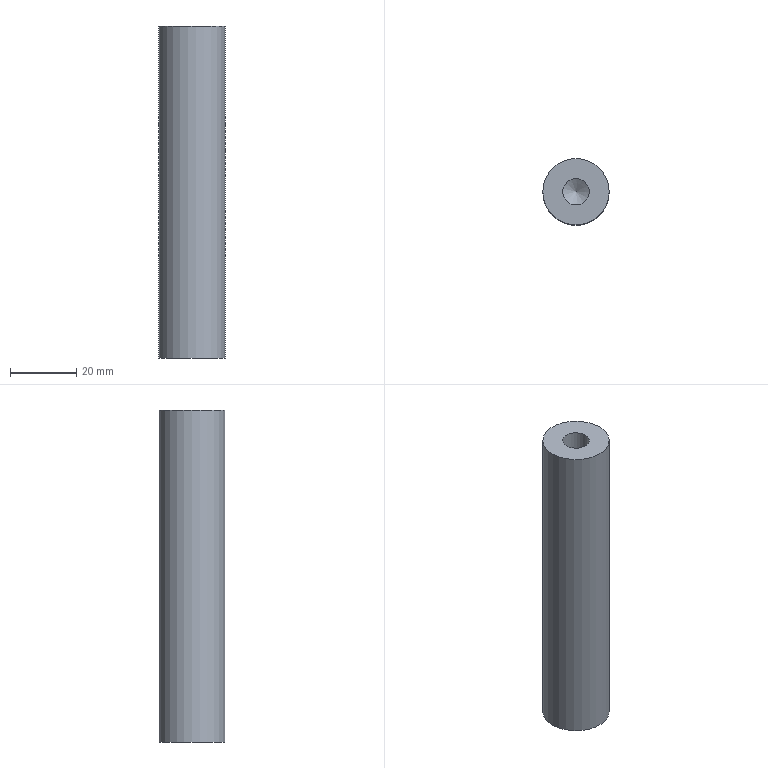Part | NX | features solid 2 | 1 solid | 7 faces | box 20 x 20 x 100 mm | volume 27520 mm3 | cylinder 3 | plane 2 | cone 2 | commonest cylinder face diameters 8 x1 12 x1 20 x1
STEP:
#1=CARTESIAN_POINT('',(-10.,-245.,5.));
#2=VERTEX_POINT('',#1);
#3=CARTESIAN_POINT('',(0.,-245.,5.));
#4=DIRECTION('',(0.,0.,-1.));
#5=DIRECTION('',(-1.,0.,0.));
#6=AXIS2_PLACEMENT_3D('',#3,#4,#5);
#7=CIRCLE('',#6,10.);
#8=EDGE_CURVE('',#2,#2,#7,.F.);
#9=ORIENTED_EDGE('',*,*,#8,.F.);
#10=EDGE_LOOP('',(#9));
#11=FACE_BOUND('',#10,.T.);
#12=CARTESIAN_POINT('',(-10.,-245.,-95.));
#13=VERTEX_POINT('',#12);
#14=CARTESIAN_POINT('',(0.,-245.,-95.));
#15=DIRECTION('',(0.,0.,-1.));
#16=DIRECTION('',(-1.,0.,0.));
#17=AXIS2_PLACEMENT_3D('',#14,#15,#16);
#18=CIRCLE('',#17,10.);
#19=EDGE_CURVE('',#13,#13,#18,.T.);
#20=ORIENTED_EDGE('',*,*,#19,.F.);
#21=EDGE_LOOP('',(#20));
#22=FACE_BOUND('',#21,.T.);
#23=CARTESIAN_POINT('',(0.,-245.,-37.));
#24=DIRECTION('',(0.,0.,1.));
#25=DIRECTION('',(0.,1.,0.));
#26=AXIS2_PLACEMENT_3D('',#23,#24,#25);
#27=CYLINDRICAL_SURFACE('',#26,10.);
#28=ADVANCED_FACE('',(#11,#22),#27,.T.);
#29=CARTESIAN_POINT('',(-6.,-245.,-95.));
#30=VERTEX_POINT('',#29);
#31=CARTESIAN_POINT('',(0.,-245.,-95.));
#32=DIRECTION('',(0.,0.,1.));
#33=DIRECTION('',(-1.,0.,0.));
#34=AXIS2_PLACEMENT_3D('',#31,#32,#33);
#35=CIRCLE('',#34,6.);
#36=EDGE_CURVE('',#30,#30,#35,.T.);
#37=ORIENTED_EDGE('',*,*,#36,.T.);
#38=EDGE_LOOP('',(#37));
#39=FACE_BOUND('',#38,.T.);
#40=ORIENTED_EDGE('',*,*,#19,.T.);
#41=EDGE_LOOP('',(#40));
#42=FACE_BOUND('',#41,.T.);
#43=CARTESIAN_POINT('',(0.,-245.,-95.));
#44=DIRECTION('',(0.,0.,-1.));
#45=DIRECTION('',(0.,-1.,0.));
#46=AXIS2_PLACEMENT_3D('',#43,#44,#45);
#47=PLANE('',#46);
#48=ADVANCED_FACE('',(#39,#42),#47,.T.);
#49=CARTESIAN_POINT('',(-6.,-245.,-71.));
#50=VERTEX_POINT('',#49);
#51=CARTESIAN_POINT('',(0.,-245.,-71.));
#52=DIRECTION('',(0.,0.,1.));
#53=DIRECTION('',(-1.,0.,0.));
#54=AXIS2_PLACEMENT_3D('',#51,#52,#53);
#55=CIRCLE('',#54,6.);
#56=EDGE_CURVE('',#50,#50,#55,.T.);
#57=ORIENTED_EDGE('',*,*,#56,.F.);
#58=EDGE_LOOP('',(#57));
#59=FACE_BOUND('',#58,.T.);
#60=CARTESIAN_POINT('',(0.,-245.,-67.395));
#61=VERTEX_POINT('',#60);
#62=VERTEX_LOOP('',#61);
#63=FACE_BOUND('',#62,.T.);
#64=CARTESIAN_POINT('',(0.,-245.,-71.));
#65=DIRECTION('',(0.,0.,-1.));
#66=DIRECTION('',(1.,0.,0.));
#67=AXIS2_PLACEMENT_3D('',#64,#65,#66);
#68=CONICAL_SURFACE('',#67,6.,1.03);
#69=ADVANCED_FACE('',(#59,#63),#68,.F.);
#70=ORIENTED_EDGE('',*,*,#56,.T.);
#71=EDGE_LOOP('',(#70));
#72=FACE_BOUND('',#71,.T.);
#73=ORIENTED_EDGE('',*,*,#36,.F.);
#74=EDGE_LOOP('',(#73));
#75=FACE_BOUND('',#74,.T.);
#76=CARTESIAN_POINT('',(0.,-245.,-85.));
#77=DIRECTION('',(0.,0.,1.));
#78=DIRECTION('',(-1.,0.,0.));
#79=AXIS2_PLACEMENT_3D('',#76,#77,#78);
#80=CYLINDRICAL_SURFACE('',#79,6.);
#81=ADVANCED_FACE('',(#72,#75),#80,.F.);
#82=CARTESIAN_POINT('',(-4.,-245.,5.));
#83=VERTEX_POINT('',#82);
#84=CARTESIAN_POINT('',(0.,-245.,5.));
#85=DIRECTION('',(0.,0.,-1.));
#86=DIRECTION('',(-1.,0.,0.));
#87=AXIS2_PLACEMENT_3D('',#84,#85,#86);
#88=CIRCLE('',#87,4.);
#89=EDGE_CURVE('',#83,#83,#88,.T.);
#90=ORIENTED_EDGE('',*,*,#89,.T.);
#91=EDGE_LOOP('',(#90));
#92=FACE_BOUND('',#91,.T.);
#93=ORIENTED_EDGE('',*,*,#8,.T.);
#94=EDGE_LOOP('',(#93));
#95=FACE_BOUND('',#94,.T.);
#96=CARTESIAN_POINT('',(0.,-245.,5.));
#97=DIRECTION('',(0.,0.,-1.));
#98=DIRECTION('',(-1.,0.,0.));
#99=AXIS2_PLACEMENT_3D('',#96,#97,#98);
#100=PLANE('',#99);
#101=ADVANCED_FACE('',(#92,#95),#100,.F.);
#102=CARTESIAN_POINT('',(-4.,-245.,-15.));
#103=VERTEX_POINT('',#102);
#104=CARTESIAN_POINT('',(0.,-245.,-15.));
#105=DIRECTION('',(0.,0.,-1.));
#106=DIRECTION('',(-1.,0.,0.));
#107=AXIS2_PLACEMENT_3D('',#104,#105,#106);
#108=CIRCLE('',#107,4.);
#109=EDGE_CURVE('',#103,#103,#108,.T.);
#110=ORIENTED_EDGE('',*,*,#109,.F.);
#111=EDGE_LOOP('',(#110));
#112=FACE_BOUND('',#111,.T.);
#113=CARTESIAN_POINT('',(0.,-245.,-17.403));
#114=VERTEX_POINT('',#113);
#115=VERTEX_LOOP('',#114);
#116=FACE_BOUND('',#115,.T.);
#117=CARTESIAN_POINT('',(0.,-245.,-15.));
#118=DIRECTION('',(0.,0.,1.));
#119=DIRECTION('',(1.,0.,0.));
#120=AXIS2_PLACEMENT_3D('',#117,#118,#119);
#121=CONICAL_SURFACE('',#120,4.,1.03);
#122=ADVANCED_FACE('',(#112,#116),#121,.F.);
#123=ORIENTED_EDGE('',*,*,#109,.T.);
#124=EDGE_LOOP('',(#123));
#125=FACE_BOUND('',#124,.T.);
#126=ORIENTED_EDGE('',*,*,#89,.F.);
#127=EDGE_LOOP('',(#126));
#128=FACE_BOUND('',#127,.T.);
#129=CARTESIAN_POINT('',(0.,-245.,5.));
#130=DIRECTION('',(0.,0.,-1.));
#131=DIRECTION('',(-1.,0.,0.));
#132=AXIS2_PLACEMENT_3D('',#129,#130,#131);
#133=CYLINDRICAL_SURFACE('',#132,4.);
#134=ADVANCED_FACE('',(#125,#128),#133,.F.);
#135=CLOSED_SHELL('',(#28,#48,#69,#81,#101,#122,#134));
#136=MANIFOLD_SOLID_BREP('',#135);
#137=(LENGTH_UNIT()NAMED_UNIT(*)SI_UNIT(.MILLI.,.METRE.));
#138=UNCERTAINTY_MEASURE_WITH_UNIT(LENGTH_MEASURE(0.00001),#137,'','');
#139=(NAMED_UNIT(*)PLANE_ANGLE_UNIT()SI_UNIT($,.RADIAN.));
#140=(NAMED_UNIT(*)SI_UNIT($,.STERADIAN.)SOLID_ANGLE_UNIT());
#141=(GEOMETRIC_REPRESENTATION_CONTEXT(3)GLOBAL_UNCERTAINTY_ASSIGNED_CONTEXT((#138))GLOBAL_UNIT_ASSIGNED_CONTEXT((#137,#139,#140))REPRESENTATION_CONTEXT('',''));
#142=ADVANCED_BREP_SHAPE_REPRESENTATION('',(#136),#141);